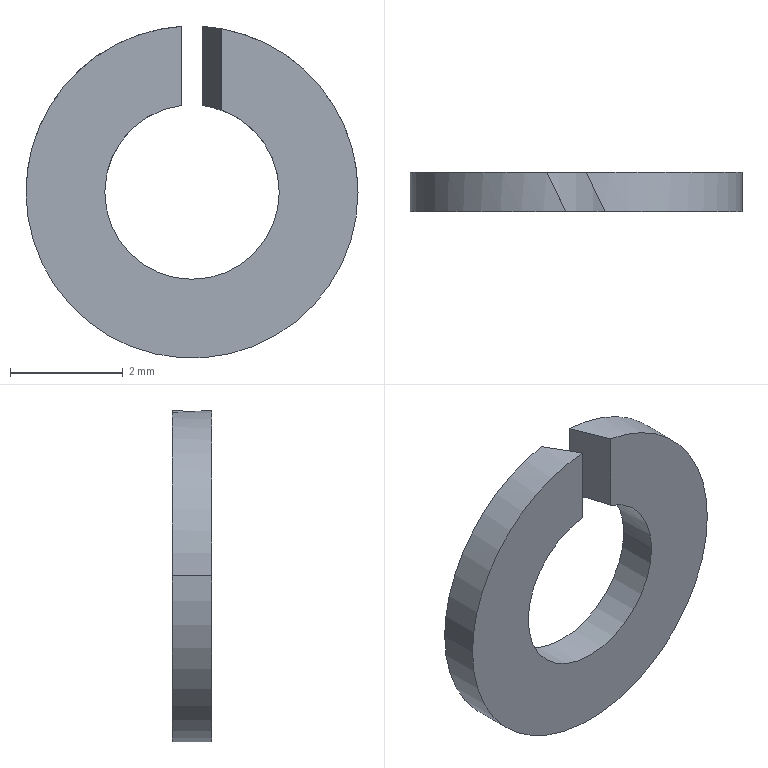Part | STEP file | ZZ24-M3-21 | 1 solid | 10 faces | box 5.9 x 0.7 x 5.895 mm | volume 13.165 mm3 | cylinder 6 | plane 4 | commonest cylinder face diameters 3.1 x3 5.9 x3
STEP:
#1=CARTESIAN_POINT('',(1.55,0.7,-0.002344));
#2=VERTEX_POINT('',#1);
#3=CARTESIAN_POINT('',(0.1793,0.7,1.54));
#4=VERTEX_POINT('',#3);
#5=CARTESIAN_POINT('',(0.,0.7,0.));
#6=DIRECTION('',(0.,-1.,0.));
#7=DIRECTION('',(-1.,0.,0.001512));
#8=AXIS2_PLACEMENT_3D('',#5,#6,#7);
#9=CIRCLE('',#8,1.55);
#10=EDGE_CURVE('',#2,#4,#9,.T.);
#11=ORIENTED_EDGE('',*,*,#10,.F.);
#12=CARTESIAN_POINT('',(1.55,0.,-0.002344));
#13=VERTEX_POINT('',#12);
#14=CARTESIAN_POINT('',(1.55,0.7,-0.002344));
#15=DIRECTION('',(0.,-1.,0.));
#16=VECTOR('',#15,1000.);
#17=LINE('',#14,#16);
#18=EDGE_CURVE('',#2,#13,#17,.T.);
#19=ORIENTED_EDGE('',*,*,#18,.T.);
#20=CARTESIAN_POINT('',(0.5207,0.,1.46));
#21=VERTEX_POINT('',#20);
#22=CARTESIAN_POINT('',(0.,0.,0.));
#23=DIRECTION('',(0.,1.,0.));
#24=DIRECTION('',(1.,0.,-0.001512));
#25=AXIS2_PLACEMENT_3D('',#22,#23,#24);
#26=CIRCLE('',#25,1.55);
#27=EDGE_CURVE('',#21,#13,#26,.T.);
#28=ORIENTED_EDGE('',*,*,#27,.F.);
#29=CARTESIAN_POINT('',(0.5207,0.,1.46));
#30=CARTESIAN_POINT('',(0.4102,0.2266,1.499));
#31=CARTESIAN_POINT('',(0.2959,0.461,1.526));
#32=CARTESIAN_POINT('',(0.1793,0.7,1.54));
#33=(BOUNDED_CURVE()B_SPLINE_CURVE(3,(#29,#30,#31,#32),.UNSPECIFIED.,.F.,.F.)B_SPLINE_CURVE_WITH_KNOTS((4,4),(1.228,1.455),.UNSPECIFIED.)CURVE()GEOMETRIC_REPRESENTATION_ITEM()RATIONAL_B_SPLINE_CURVE((1.,0.9957,0.9957,1.))REPRESENTATION_ITEM(''));
#34=EDGE_CURVE('',#21,#4,#33,.T.);
#35=ORIENTED_EDGE('',*,*,#34,.T.);
#36=EDGE_LOOP('',(#11,#19,#28,#35));
#37=FACE_OUTER_BOUND('',#36,.T.);
#38=CARTESIAN_POINT('',(0.,0.7,0.));
#39=DIRECTION('',(0.,-1.,0.));
#40=DIRECTION('',(-1.,0.,0.001512));
#41=AXIS2_PLACEMENT_3D('',#38,#39,#40);
#42=CYLINDRICAL_SURFACE('',#41,1.55);
#43=ADVANCED_FACE('',(#37),#42,.F.);
#44=ORIENTED_EDGE('',*,*,#18,.F.);
#45=CARTESIAN_POINT('',(-1.55,0.7,0.002344));
#46=VERTEX_POINT('',#45);
#47=CARTESIAN_POINT('',(0.,0.7,0.));
#48=DIRECTION('',(0.,-1.,0.));
#49=DIRECTION('',(-1.,0.,0.001512));
#50=AXIS2_PLACEMENT_3D('',#47,#48,#49);
#51=CIRCLE('',#50,1.55);
#52=EDGE_CURVE('',#46,#2,#51,.T.);
#53=ORIENTED_EDGE('',*,*,#52,.F.);
#54=CARTESIAN_POINT('',(-1.55,0.,0.002344));
#55=VERTEX_POINT('',#54);
#56=CARTESIAN_POINT('',(-1.55,0.7,0.002344));
#57=DIRECTION('',(0.,-1.,0.));
#58=VECTOR('',#57,1000.);
#59=LINE('',#56,#58);
#60=EDGE_CURVE('',#46,#55,#59,.T.);
#61=ORIENTED_EDGE('',*,*,#60,.T.);
#62=CARTESIAN_POINT('',(0.,0.,0.));
#63=DIRECTION('',(0.,1.,0.));
#64=DIRECTION('',(1.,0.,-0.001512));
#65=AXIS2_PLACEMENT_3D('',#62,#63,#64);
#66=CIRCLE('',#65,1.55);
#67=EDGE_CURVE('',#13,#55,#66,.T.);
#68=ORIENTED_EDGE('',*,*,#67,.F.);
#69=EDGE_LOOP('',(#44,#53,#61,#68));
#70=FACE_OUTER_BOUND('',#69,.T.);
#71=CARTESIAN_POINT('',(0.,0.7,0.));
#72=DIRECTION('',(0.,-1.,0.));
#73=DIRECTION('',(-1.,0.,0.001512));
#74=AXIS2_PLACEMENT_3D('',#71,#72,#73);
#75=CYLINDRICAL_SURFACE('',#74,1.55);
#76=ADVANCED_FACE('',(#70),#75,.F.);
#77=CARTESIAN_POINT('',(-2.95,0.7,0.004461));
#78=VERTEX_POINT('',#77);
#79=CARTESIAN_POINT('',(2.95,0.7,-0.004461));
#80=VERTEX_POINT('',#79);
#81=CARTESIAN_POINT('',(0.,0.7,0.));
#82=DIRECTION('',(0.,-1.,0.));
#83=DIRECTION('',(-1.,0.,0.001512));
#84=AXIS2_PLACEMENT_3D('',#81,#82,#83);
#85=CIRCLE('',#84,2.95);
#86=EDGE_CURVE('',#78,#80,#85,.T.);
#87=ORIENTED_EDGE('',*,*,#86,.T.);
#88=CARTESIAN_POINT('',(2.95,0.,-0.004461));
#89=VERTEX_POINT('',#88);
#90=CARTESIAN_POINT('',(2.95,0.7,-0.004461));
#91=DIRECTION('',(0.,-1.,0.));
#92=VECTOR('',#91,1000.);
#93=LINE('',#90,#92);
#94=EDGE_CURVE('',#80,#89,#93,.T.);
#95=ORIENTED_EDGE('',*,*,#94,.T.);
#96=CARTESIAN_POINT('',(-2.95,0.,0.004461));
#97=VERTEX_POINT('',#96);
#98=CARTESIAN_POINT('',(0.,0.,0.));
#99=DIRECTION('',(0.,1.,0.));
#100=DIRECTION('',(1.,0.,-0.001512));
#101=AXIS2_PLACEMENT_3D('',#98,#99,#100);
#102=CIRCLE('',#101,2.95);
#103=EDGE_CURVE('',#89,#97,#102,.T.);
#104=ORIENTED_EDGE('',*,*,#103,.T.);
#105=CARTESIAN_POINT('',(-2.95,0.7,0.004461));
#106=DIRECTION('',(0.,-1.,0.));
#107=VECTOR('',#106,1000.);
#108=LINE('',#105,#107);
#109=EDGE_CURVE('',#78,#97,#108,.T.);
#110=ORIENTED_EDGE('',*,*,#109,.F.);
#111=EDGE_LOOP('',(#87,#95,#104,#110));
#112=FACE_OUTER_BOUND('',#111,.T.);
#113=CARTESIAN_POINT('',(0.,0.7,0.));
#114=DIRECTION('',(0.,-1.,0.));
#115=DIRECTION('',(-1.,0.,0.001512));
#116=AXIS2_PLACEMENT_3D('',#113,#114,#115);
#117=CYLINDRICAL_SURFACE('',#116,2.95);
#118=ADVANCED_FACE('',(#112),#117,.T.);
#119=CARTESIAN_POINT('',(-0.5207,0.7,2.904));
#120=VERTEX_POINT('',#119);
#121=CARTESIAN_POINT('',(0.,0.7,0.));
#122=DIRECTION('',(0.,-1.,0.));
#123=DIRECTION('',(-1.,0.,0.001512));
#124=AXIS2_PLACEMENT_3D('',#121,#122,#123);
#125=CIRCLE('',#124,2.95);
#126=EDGE_CURVE('',#120,#78,#125,.T.);
#127=ORIENTED_EDGE('',*,*,#126,.T.);
#128=ORIENTED_EDGE('',*,*,#109,.T.);
#129=CARTESIAN_POINT('',(-0.1793,0.,2.945));
#130=VERTEX_POINT('',#129);
#131=CARTESIAN_POINT('',(0.,0.,0.));
#132=DIRECTION('',(0.,1.,0.));
#133=DIRECTION('',(1.,0.,-0.001512));
#134=AXIS2_PLACEMENT_3D('',#131,#132,#133);
#135=CIRCLE('',#134,2.95);
#136=EDGE_CURVE('',#97,#130,#135,.T.);
#137=ORIENTED_EDGE('',*,*,#136,.T.);
#138=CARTESIAN_POINT('',(-0.1793,0.,2.945));
#139=CARTESIAN_POINT('',(-0.2938,0.2348,2.938));
#140=CARTESIAN_POINT('',(-0.4078,0.4684,2.924));
#141=CARTESIAN_POINT('',(-0.5207,0.7,2.904));
#142=(BOUNDED_CURVE()B_SPLINE_CURVE(3,(#138,#139,#140,#141),.UNSPECIFIED.,.F.,.F.)B_SPLINE_CURVE_WITH_KNOTS((4,4),(1.632,1.748),.UNSPECIFIED.)CURVE()GEOMETRIC_REPRESENTATION_ITEM()RATIONAL_B_SPLINE_CURVE((1.,0.9989,0.9989,1.))REPRESENTATION_ITEM(''));
#143=EDGE_CURVE('',#130,#120,#142,.T.);
#144=ORIENTED_EDGE('',*,*,#143,.T.);
#145=EDGE_LOOP('',(#127,#128,#137,#144));
#146=FACE_OUTER_BOUND('',#145,.T.);
#147=CARTESIAN_POINT('',(0.,0.7,0.));
#148=DIRECTION('',(0.,-1.,0.));
#149=DIRECTION('',(-1.,0.,0.001512));
#150=AXIS2_PLACEMENT_3D('',#147,#148,#149);
#151=CYLINDRICAL_SURFACE('',#150,2.95);
#152=ADVANCED_FACE('',(#146),#151,.T.);
#153=CARTESIAN_POINT('',(-0.1793,0.,1.54));
#154=VERTEX_POINT('',#153);
#155=CARTESIAN_POINT('',(-0.1793,0.,2.95));
#156=DIRECTION('',(0.,0.,-1.));
#157=VECTOR('',#156,1000.);
#158=LINE('',#155,#157);
#159=EDGE_CURVE('',#130,#154,#158,.T.);
#160=ORIENTED_EDGE('',*,*,#159,.F.);
#161=ORIENTED_EDGE('',*,*,#136,.F.);
#162=ORIENTED_EDGE('',*,*,#103,.F.);
#163=CARTESIAN_POINT('',(0.5207,0.,2.904));
#164=VERTEX_POINT('',#163);
#165=CARTESIAN_POINT('',(0.,0.,0.));
#166=DIRECTION('',(0.,1.,0.));
#167=DIRECTION('',(1.,0.,-0.001512));
#168=AXIS2_PLACEMENT_3D('',#165,#166,#167);
#169=CIRCLE('',#168,2.95);
#170=EDGE_CURVE('',#164,#89,#169,.T.);
#171=ORIENTED_EDGE('',*,*,#170,.F.);
#172=CARTESIAN_POINT('',(0.5207,0.,2.95));
#173=DIRECTION('',(0.,0.,-1.));
#174=VECTOR('',#173,1000.);
#175=LINE('',#172,#174);
#176=EDGE_CURVE('',#164,#21,#175,.T.);
#177=ORIENTED_EDGE('',*,*,#176,.T.);
#178=ORIENTED_EDGE('',*,*,#27,.T.);
#179=ORIENTED_EDGE('',*,*,#67,.T.);
#180=CARTESIAN_POINT('',(0.,0.,0.));
#181=DIRECTION('',(0.,1.,0.));
#182=DIRECTION('',(1.,0.,-0.001512));
#183=AXIS2_PLACEMENT_3D('',#180,#181,#182);
#184=CIRCLE('',#183,1.55);
#185=EDGE_CURVE('',#55,#154,#184,.T.);
#186=ORIENTED_EDGE('',*,*,#185,.T.);
#187=EDGE_LOOP('',(#160,#161,#162,#171,#177,#178,#179,#186));
#188=FACE_OUTER_BOUND('',#187,.T.);
#189=CARTESIAN_POINT('',(0.,0.,0.));
#190=DIRECTION('',(0.,-1.,0.));
#191=DIRECTION('',(-1.,0.,0.001512));
#192=AXIS2_PLACEMENT_3D('',#189,#190,#191);
#193=PLANE('',#192);
#194=ADVANCED_FACE('',(#188),#193,.T.);
#195=CARTESIAN_POINT('',(0.1793,0.7,2.945));
#196=VERTEX_POINT('',#195);
#197=CARTESIAN_POINT('',(0.1793,0.7,2.95));
#198=DIRECTION('',(0.,0.,-1.));
#199=VECTOR('',#198,1000.);
#200=LINE('',#197,#199);
#201=EDGE_CURVE('',#196,#4,#200,.T.);
#202=ORIENTED_EDGE('',*,*,#201,.F.);
#203=CARTESIAN_POINT('',(0.,0.7,0.));
#204=DIRECTION('',(0.,-1.,0.));
#205=DIRECTION('',(-1.,0.,0.001512));
#206=AXIS2_PLACEMENT_3D('',#203,#204,#205);
#207=CIRCLE('',#206,2.95);
#208=EDGE_CURVE('',#80,#196,#207,.T.);
#209=ORIENTED_EDGE('',*,*,#208,.F.);
#210=ORIENTED_EDGE('',*,*,#86,.F.);
#211=ORIENTED_EDGE('',*,*,#126,.F.);
#212=CARTESIAN_POINT('',(-0.5207,0.7,1.46));
#213=VERTEX_POINT('',#212);
#214=CARTESIAN_POINT('',(-0.5207,0.7,2.95));
#215=DIRECTION('',(0.,0.,-1.));
#216=VECTOR('',#215,1000.);
#217=LINE('',#214,#216);
#218=EDGE_CURVE('',#120,#213,#217,.T.);
#219=ORIENTED_EDGE('',*,*,#218,.T.);
#220=CARTESIAN_POINT('',(0.,0.7,0.));
#221=DIRECTION('',(0.,-1.,0.));
#222=DIRECTION('',(-1.,0.,0.001512));
#223=AXIS2_PLACEMENT_3D('',#220,#221,#222);
#224=CIRCLE('',#223,1.55);
#225=EDGE_CURVE('',#213,#46,#224,.T.);
#226=ORIENTED_EDGE('',*,*,#225,.T.);
#227=ORIENTED_EDGE('',*,*,#52,.T.);
#228=ORIENTED_EDGE('',*,*,#10,.T.);
#229=EDGE_LOOP('',(#202,#209,#210,#211,#219,#226,#227,#228));
#230=FACE_OUTER_BOUND('',#229,.T.);
#231=CARTESIAN_POINT('',(0.,0.7,0.));
#232=DIRECTION('',(0.,1.,0.));
#233=DIRECTION('',(1.,0.,-0.001512));
#234=AXIS2_PLACEMENT_3D('',#231,#232,#233);
#235=PLANE('',#234);
#236=ADVANCED_FACE('',(#230),#235,.T.);
#237=ORIENTED_EDGE('',*,*,#94,.F.);
#238=ORIENTED_EDGE('',*,*,#208,.T.);
#239=CARTESIAN_POINT('',(0.1793,0.7,2.945));
#240=CARTESIAN_POINT('',(0.2938,0.4652,2.938));
#241=CARTESIAN_POINT('',(0.4078,0.2316,2.924));
#242=CARTESIAN_POINT('',(0.5207,0.,2.904));
#243=(BOUNDED_CURVE()B_SPLINE_CURVE(3,(#239,#240,#241,#242),.UNSPECIFIED.,.F.,.F.)B_SPLINE_CURVE_WITH_KNOTS((4,4),(4.773,4.89),.UNSPECIFIED.)CURVE()GEOMETRIC_REPRESENTATION_ITEM()RATIONAL_B_SPLINE_CURVE((1.,0.9989,0.9989,1.))REPRESENTATION_ITEM(''));
#244=EDGE_CURVE('',#196,#164,#243,.T.);
#245=ORIENTED_EDGE('',*,*,#244,.T.);
#246=ORIENTED_EDGE('',*,*,#170,.T.);
#247=EDGE_LOOP('',(#237,#238,#245,#246));
#248=FACE_OUTER_BOUND('',#247,.T.);
#249=CARTESIAN_POINT('',(0.,0.7,0.));
#250=DIRECTION('',(0.,-1.,0.));
#251=DIRECTION('',(-1.,0.,0.001512));
#252=AXIS2_PLACEMENT_3D('',#249,#250,#251);
#253=CYLINDRICAL_SURFACE('',#252,2.95);
#254=ADVANCED_FACE('',(#248),#253,.T.);
#255=ORIENTED_EDGE('',*,*,#201,.T.);
#256=ORIENTED_EDGE('',*,*,#34,.F.);
#257=ORIENTED_EDGE('',*,*,#176,.F.);
#258=ORIENTED_EDGE('',*,*,#244,.F.);
#259=EDGE_LOOP('',(#255,#256,#257,#258));
#260=FACE_OUTER_BOUND('',#259,.T.);
#261=CARTESIAN_POINT('',(0.5207,0.,2.95));
#262=DIRECTION('',(-0.8988,-0.4384,0.));
#263=DIRECTION('',(0.4384,-0.8988,0.));
#264=AXIS2_PLACEMENT_3D('',#261,#262,#263);
#265=PLANE('',#264);
#266=ADVANCED_FACE('',(#260),#265,.T.);
#267=ORIENTED_EDGE('',*,*,#159,.T.);
#268=CARTESIAN_POINT('',(-0.5207,0.7,1.46));
#269=CARTESIAN_POINT('',(-0.4102,0.4734,1.499));
#270=CARTESIAN_POINT('',(-0.2959,0.239,1.526));
#271=CARTESIAN_POINT('',(-0.1793,0.,1.54));
#272=(BOUNDED_CURVE()B_SPLINE_CURVE(3,(#268,#269,#270,#271),.UNSPECIFIED.,.F.,.F.)B_SPLINE_CURVE_WITH_KNOTS((4,4),(4.37,4.596),.UNSPECIFIED.)CURVE()GEOMETRIC_REPRESENTATION_ITEM()RATIONAL_B_SPLINE_CURVE((1.,0.9957,0.9957,1.))REPRESENTATION_ITEM(''));
#273=EDGE_CURVE('',#213,#154,#272,.T.);
#274=ORIENTED_EDGE('',*,*,#273,.F.);
#275=ORIENTED_EDGE('',*,*,#218,.F.);
#276=ORIENTED_EDGE('',*,*,#143,.F.);
#277=EDGE_LOOP('',(#267,#274,#275,#276));
#278=FACE_OUTER_BOUND('',#277,.T.);
#279=CARTESIAN_POINT('',(-0.5207,0.7,2.95));
#280=DIRECTION('',(0.8988,0.4384,0.));
#281=DIRECTION('',(-0.4384,0.8988,0.));
#282=AXIS2_PLACEMENT_3D('',#279,#280,#281);
#283=PLANE('',#282);
#284=ADVANCED_FACE('',(#278),#283,.T.);
#285=ORIENTED_EDGE('',*,*,#60,.F.);
#286=ORIENTED_EDGE('',*,*,#225,.F.);
#287=ORIENTED_EDGE('',*,*,#273,.T.);
#288=ORIENTED_EDGE('',*,*,#185,.F.);
#289=EDGE_LOOP('',(#285,#286,#287,#288));
#290=FACE_OUTER_BOUND('',#289,.T.);
#291=CARTESIAN_POINT('',(0.,0.7,0.));
#292=DIRECTION('',(0.,-1.,0.));
#293=DIRECTION('',(-1.,0.,0.001512));
#294=AXIS2_PLACEMENT_3D('',#291,#292,#293);
#295=CYLINDRICAL_SURFACE('',#294,1.55);
#296=ADVANCED_FACE('',(#290),#295,.F.);
#297=CLOSED_SHELL('',(#43,#76,#118,#152,#194,#236,#254,#266,#284,#296));
#298=MANIFOLD_SOLID_BREP('',#297);
#299=CARTESIAN_POINT('',(0.,0.,0.));
#300=DIRECTION('',(0.,0.,1.));
#301=DIRECTION('',(1.,0.,0.));
#302=AXIS2_PLACEMENT_3D('',#299,#300,#301);
#303=(LENGTH_UNIT()NAMED_UNIT(*)SI_UNIT(.MILLI.,.METRE.));
#304=UNCERTAINTY_MEASURE_WITH_UNIT(LENGTH_MEASURE(0.00001),#303,'','');
#305=(NAMED_UNIT(*)PLANE_ANGLE_UNIT()SI_UNIT($,.RADIAN.));
#306=(NAMED_UNIT(*)SI_UNIT($,.STERADIAN.)SOLID_ANGLE_UNIT());
#307=(GEOMETRIC_REPRESENTATION_CONTEXT(3)GLOBAL_UNCERTAINTY_ASSIGNED_CONTEXT((#304))GLOBAL_UNIT_ASSIGNED_CONTEXT((#303,#305,#306))REPRESENTATION_CONTEXT('',''));
#308=ADVANCED_BREP_SHAPE_REPRESENTATION('',(#298,#302),#307);